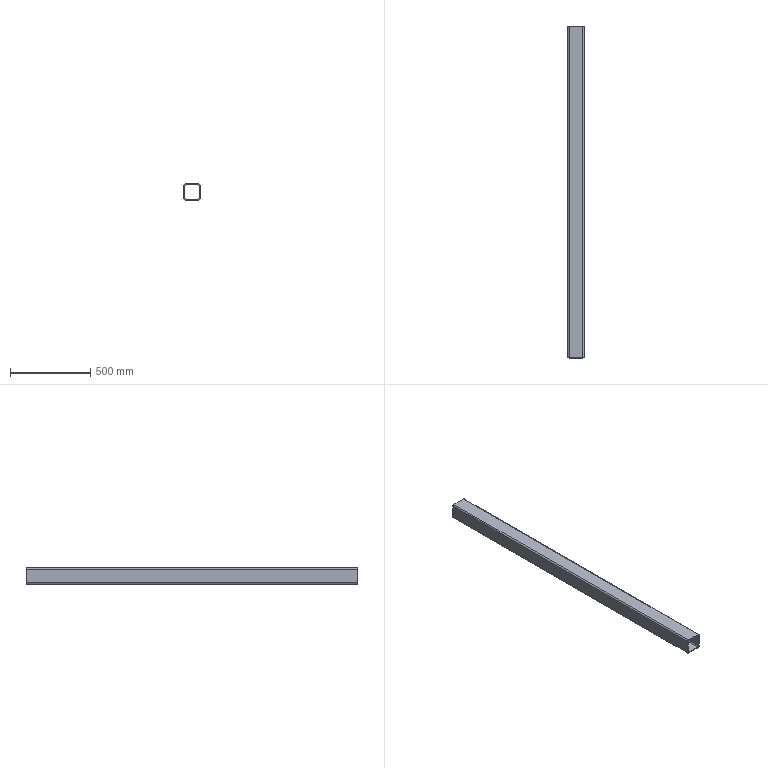Part | SolidWorks | features Extrusion 1 | 1 solid | 18 faces | box 100 x 2070 x 100 mm | volume 4848096 mm3 | plane 10 | cylinder 8 | commonest cylinder face diameters 12.6 x4 15.75 x4
STEP:
#1=CARTESIAN_POINT('',(100.,2070.,-90.6));
#2=VERTEX_POINT('',#1);
#3=CARTESIAN_POINT('',(92.125,2070.,-98.475));
#4=VERTEX_POINT('',#3);
#5=CARTESIAN_POINT('',(92.125,2070.,-90.6));
#6=DIRECTION('',(0.,1.,0.));
#7=DIRECTION('',(0.,0.,1.));
#8=AXIS2_PLACEMENT_3D('',#5,#6,#7);
#9=CIRCLE('',#8,7.875);
#10=EDGE_CURVE('',#2,#4,#9,.T.);
#11=ORIENTED_EDGE('',*,*,#10,.T.);
#12=CARTESIAN_POINT('',(7.875,2070.,-98.475));
#13=VERTEX_POINT('',#12);
#14=CARTESIAN_POINT('',(92.125,2070.,-98.475));
#15=DIRECTION('',(-1.,0.,0.));
#16=VECTOR('',#15,1000.);
#17=LINE('',#14,#16);
#18=EDGE_CURVE('',#4,#13,#17,.T.);
#19=ORIENTED_EDGE('',*,*,#18,.T.);
#20=CARTESIAN_POINT('',(0.,2070.,-90.6));
#21=VERTEX_POINT('',#20);
#22=CARTESIAN_POINT('',(7.875,2070.,-90.6));
#23=DIRECTION('',(0.,1.,0.));
#24=DIRECTION('',(0.,0.,1.));
#25=AXIS2_PLACEMENT_3D('',#22,#23,#24);
#26=CIRCLE('',#25,7.875);
#27=EDGE_CURVE('',#13,#21,#26,.T.);
#28=ORIENTED_EDGE('',*,*,#27,.T.);
#29=CARTESIAN_POINT('',(0.,2070.,-6.35));
#30=VERTEX_POINT('',#29);
#31=CARTESIAN_POINT('',(0.,2070.,-6.35));
#32=DIRECTION('',(0.,0.,1.));
#33=VECTOR('',#32,1000.);
#34=LINE('',#31,#33);
#35=EDGE_CURVE('',#21,#30,#34,.T.);
#36=ORIENTED_EDGE('',*,*,#35,.T.);
#37=CARTESIAN_POINT('',(7.875,2070.,1.525));
#38=VERTEX_POINT('',#37);
#39=CARTESIAN_POINT('',(7.875,2070.,-6.35));
#40=DIRECTION('',(0.,1.,0.));
#41=DIRECTION('',(0.,0.,1.));
#42=AXIS2_PLACEMENT_3D('',#39,#40,#41);
#43=CIRCLE('',#42,7.875);
#44=EDGE_CURVE('',#30,#38,#43,.T.);
#45=ORIENTED_EDGE('',*,*,#44,.T.);
#46=CARTESIAN_POINT('',(92.125,2070.,1.525));
#47=VERTEX_POINT('',#46);
#48=CARTESIAN_POINT('',(7.875,2070.,1.525));
#49=DIRECTION('',(1.,0.,0.));
#50=VECTOR('',#49,1000.);
#51=LINE('',#48,#50);
#52=EDGE_CURVE('',#38,#47,#51,.T.);
#53=ORIENTED_EDGE('',*,*,#52,.T.);
#54=CARTESIAN_POINT('',(100.,2070.,-6.35));
#55=VERTEX_POINT('',#54);
#56=CARTESIAN_POINT('',(92.125,2070.,-6.35));
#57=DIRECTION('',(0.,1.,0.));
#58=DIRECTION('',(0.,0.,1.));
#59=AXIS2_PLACEMENT_3D('',#56,#57,#58);
#60=CIRCLE('',#59,7.875);
#61=EDGE_CURVE('',#47,#55,#60,.T.);
#62=ORIENTED_EDGE('',*,*,#61,.T.);
#63=CARTESIAN_POINT('',(100.,2070.,-90.6));
#64=DIRECTION('',(0.,0.,-1.));
#65=VECTOR('',#64,1000.);
#66=LINE('',#63,#65);
#67=EDGE_CURVE('',#55,#2,#66,.T.);
#68=ORIENTED_EDGE('',*,*,#67,.T.);
#69=EDGE_LOOP('',(#11,#19,#28,#36,#45,#53,#62,#68));
#70=FACE_OUTER_BOUND('',#69,.T.);
#71=CARTESIAN_POINT('',(6.3,2070.,-85.875));
#72=VERTEX_POINT('',#71);
#73=CARTESIAN_POINT('',(6.3,2070.,-11.075));
#74=VERTEX_POINT('',#73);
#75=CARTESIAN_POINT('',(6.3,2070.,-11.075));
#76=DIRECTION('',(0.,0.,1.));
#77=VECTOR('',#76,1000.);
#78=LINE('',#75,#77);
#79=EDGE_CURVE('',#72,#74,#78,.T.);
#80=ORIENTED_EDGE('',*,*,#79,.F.);
#81=CARTESIAN_POINT('',(12.6,2070.,-92.175));
#82=VERTEX_POINT('',#81);
#83=CARTESIAN_POINT('',(12.6,2070.,-85.875));
#84=DIRECTION('',(0.,1.,0.));
#85=DIRECTION('',(0.,0.,1.));
#86=AXIS2_PLACEMENT_3D('',#83,#84,#85);
#87=CIRCLE('',#86,6.3);
#88=EDGE_CURVE('',#82,#72,#87,.T.);
#89=ORIENTED_EDGE('',*,*,#88,.F.);
#90=CARTESIAN_POINT('',(87.4,2070.,-92.175));
#91=VERTEX_POINT('',#90);
#92=CARTESIAN_POINT('',(87.4,2070.,-92.175));
#93=DIRECTION('',(-1.,0.,0.));
#94=VECTOR('',#93,1000.);
#95=LINE('',#92,#94);
#96=EDGE_CURVE('',#91,#82,#95,.T.);
#97=ORIENTED_EDGE('',*,*,#96,.F.);
#98=CARTESIAN_POINT('',(93.7,2070.,-85.875));
#99=VERTEX_POINT('',#98);
#100=CARTESIAN_POINT('',(87.4,2070.,-85.875));
#101=DIRECTION('',(0.,1.,0.));
#102=DIRECTION('',(0.,0.,1.));
#103=AXIS2_PLACEMENT_3D('',#100,#101,#102);
#104=CIRCLE('',#103,6.3);
#105=EDGE_CURVE('',#99,#91,#104,.T.);
#106=ORIENTED_EDGE('',*,*,#105,.F.);
#107=CARTESIAN_POINT('',(93.7,2070.,-11.075));
#108=VERTEX_POINT('',#107);
#109=CARTESIAN_POINT('',(93.7,2070.,-85.875));
#110=DIRECTION('',(0.,0.,-1.));
#111=VECTOR('',#110,1000.);
#112=LINE('',#109,#111);
#113=EDGE_CURVE('',#108,#99,#112,.T.);
#114=ORIENTED_EDGE('',*,*,#113,.F.);
#115=CARTESIAN_POINT('',(87.4,2070.,-4.775));
#116=VERTEX_POINT('',#115);
#117=CARTESIAN_POINT('',(87.4,2070.,-11.075));
#118=DIRECTION('',(0.,1.,0.));
#119=DIRECTION('',(0.,0.,1.));
#120=AXIS2_PLACEMENT_3D('',#117,#118,#119);
#121=CIRCLE('',#120,6.3);
#122=EDGE_CURVE('',#116,#108,#121,.T.);
#123=ORIENTED_EDGE('',*,*,#122,.F.);
#124=CARTESIAN_POINT('',(12.6,2070.,-4.775));
#125=VERTEX_POINT('',#124);
#126=CARTESIAN_POINT('',(12.6,2070.,-4.775));
#127=DIRECTION('',(1.,0.,0.));
#128=VECTOR('',#127,1000.);
#129=LINE('',#126,#128);
#130=EDGE_CURVE('',#125,#116,#129,.T.);
#131=ORIENTED_EDGE('',*,*,#130,.F.);
#132=CARTESIAN_POINT('',(12.6,2070.,-11.075));
#133=DIRECTION('',(0.,1.,0.));
#134=DIRECTION('',(0.,0.,1.));
#135=AXIS2_PLACEMENT_3D('',#132,#133,#134);
#136=CIRCLE('',#135,6.3);
#137=EDGE_CURVE('',#74,#125,#136,.T.);
#138=ORIENTED_EDGE('',*,*,#137,.F.);
#139=EDGE_LOOP('',(#80,#89,#97,#106,#114,#123,#131,#138));
#140=FACE_BOUND('',#139,.T.);
#141=CARTESIAN_POINT('',(92.125,2070.,-90.6));
#142=DIRECTION('',(0.,1.,0.));
#143=DIRECTION('',(0.,0.,1.));
#144=AXIS2_PLACEMENT_3D('',#141,#142,#143);
#145=PLANE('',#144);
#146=ADVANCED_FACE('',(#70,#140),#145,.T.);
#147=CARTESIAN_POINT('',(100.,0.,-90.6));
#148=VERTEX_POINT('',#147);
#149=CARTESIAN_POINT('',(92.125,0.,-98.475));
#150=VERTEX_POINT('',#149);
#151=CARTESIAN_POINT('',(92.125,0.,-90.6));
#152=DIRECTION('',(0.,1.,0.));
#153=DIRECTION('',(0.,0.,1.));
#154=AXIS2_PLACEMENT_3D('',#151,#152,#153);
#155=CIRCLE('',#154,7.875);
#156=EDGE_CURVE('',#148,#150,#155,.T.);
#157=ORIENTED_EDGE('',*,*,#156,.F.);
#158=CARTESIAN_POINT('',(100.,0.,-6.35));
#159=VERTEX_POINT('',#158);
#160=CARTESIAN_POINT('',(100.,0.,-90.6));
#161=DIRECTION('',(0.,0.,-1.));
#162=VECTOR('',#161,1000.);
#163=LINE('',#160,#162);
#164=EDGE_CURVE('',#159,#148,#163,.T.);
#165=ORIENTED_EDGE('',*,*,#164,.F.);
#166=CARTESIAN_POINT('',(92.125,0.,1.525));
#167=VERTEX_POINT('',#166);
#168=CARTESIAN_POINT('',(92.125,0.,-6.35));
#169=DIRECTION('',(0.,1.,0.));
#170=DIRECTION('',(0.,0.,1.));
#171=AXIS2_PLACEMENT_3D('',#168,#169,#170);
#172=CIRCLE('',#171,7.875);
#173=EDGE_CURVE('',#167,#159,#172,.T.);
#174=ORIENTED_EDGE('',*,*,#173,.F.);
#175=CARTESIAN_POINT('',(7.875,0.,1.525));
#176=VERTEX_POINT('',#175);
#177=CARTESIAN_POINT('',(7.875,0.,1.525));
#178=DIRECTION('',(1.,0.,0.));
#179=VECTOR('',#178,1000.);
#180=LINE('',#177,#179);
#181=EDGE_CURVE('',#176,#167,#180,.T.);
#182=ORIENTED_EDGE('',*,*,#181,.F.);
#183=CARTESIAN_POINT('',(0.,0.,-6.35));
#184=VERTEX_POINT('',#183);
#185=CARTESIAN_POINT('',(7.875,0.,-6.35));
#186=DIRECTION('',(0.,1.,0.));
#187=DIRECTION('',(0.,0.,1.));
#188=AXIS2_PLACEMENT_3D('',#185,#186,#187);
#189=CIRCLE('',#188,7.875);
#190=EDGE_CURVE('',#184,#176,#189,.T.);
#191=ORIENTED_EDGE('',*,*,#190,.F.);
#192=CARTESIAN_POINT('',(0.,0.,-90.6));
#193=VERTEX_POINT('',#192);
#194=CARTESIAN_POINT('',(0.,0.,-6.35));
#195=DIRECTION('',(0.,0.,1.));
#196=VECTOR('',#195,1000.);
#197=LINE('',#194,#196);
#198=EDGE_CURVE('',#193,#184,#197,.T.);
#199=ORIENTED_EDGE('',*,*,#198,.F.);
#200=CARTESIAN_POINT('',(7.875,0.,-98.475));
#201=VERTEX_POINT('',#200);
#202=CARTESIAN_POINT('',(7.875,0.,-90.6));
#203=DIRECTION('',(0.,1.,0.));
#204=DIRECTION('',(0.,0.,1.));
#205=AXIS2_PLACEMENT_3D('',#202,#203,#204);
#206=CIRCLE('',#205,7.875);
#207=EDGE_CURVE('',#201,#193,#206,.T.);
#208=ORIENTED_EDGE('',*,*,#207,.F.);
#209=CARTESIAN_POINT('',(92.125,0.,-98.475));
#210=DIRECTION('',(-1.,0.,0.));
#211=VECTOR('',#210,1000.);
#212=LINE('',#209,#211);
#213=EDGE_CURVE('',#150,#201,#212,.T.);
#214=ORIENTED_EDGE('',*,*,#213,.F.);
#215=EDGE_LOOP('',(#157,#165,#174,#182,#191,#199,#208,#214));
#216=FACE_OUTER_BOUND('',#215,.T.);
#217=CARTESIAN_POINT('',(12.6,0.,-92.175));
#218=VERTEX_POINT('',#217);
#219=CARTESIAN_POINT('',(6.3,0.,-85.875));
#220=VERTEX_POINT('',#219);
#221=CARTESIAN_POINT('',(12.6,0.,-85.875));
#222=DIRECTION('',(0.,1.,0.));
#223=DIRECTION('',(0.,0.,1.));
#224=AXIS2_PLACEMENT_3D('',#221,#222,#223);
#225=CIRCLE('',#224,6.3);
#226=EDGE_CURVE('',#218,#220,#225,.T.);
#227=ORIENTED_EDGE('',*,*,#226,.T.);
#228=CARTESIAN_POINT('',(6.3,0.,-11.075));
#229=VERTEX_POINT('',#228);
#230=CARTESIAN_POINT('',(6.3,0.,-11.075));
#231=DIRECTION('',(0.,0.,1.));
#232=VECTOR('',#231,1000.);
#233=LINE('',#230,#232);
#234=EDGE_CURVE('',#220,#229,#233,.T.);
#235=ORIENTED_EDGE('',*,*,#234,.T.);
#236=CARTESIAN_POINT('',(12.6,0.,-4.775));
#237=VERTEX_POINT('',#236);
#238=CARTESIAN_POINT('',(12.6,0.,-11.075));
#239=DIRECTION('',(0.,1.,0.));
#240=DIRECTION('',(0.,0.,1.));
#241=AXIS2_PLACEMENT_3D('',#238,#239,#240);
#242=CIRCLE('',#241,6.3);
#243=EDGE_CURVE('',#229,#237,#242,.T.);
#244=ORIENTED_EDGE('',*,*,#243,.T.);
#245=CARTESIAN_POINT('',(87.4,0.,-4.775));
#246=VERTEX_POINT('',#245);
#247=CARTESIAN_POINT('',(12.6,0.,-4.775));
#248=DIRECTION('',(1.,0.,0.));
#249=VECTOR('',#248,1000.);
#250=LINE('',#247,#249);
#251=EDGE_CURVE('',#237,#246,#250,.T.);
#252=ORIENTED_EDGE('',*,*,#251,.T.);
#253=CARTESIAN_POINT('',(93.7,0.,-11.075));
#254=VERTEX_POINT('',#253);
#255=CARTESIAN_POINT('',(87.4,0.,-11.075));
#256=DIRECTION('',(0.,1.,0.));
#257=DIRECTION('',(0.,0.,1.));
#258=AXIS2_PLACEMENT_3D('',#255,#256,#257);
#259=CIRCLE('',#258,6.3);
#260=EDGE_CURVE('',#246,#254,#259,.T.);
#261=ORIENTED_EDGE('',*,*,#260,.T.);
#262=CARTESIAN_POINT('',(93.7,0.,-85.875));
#263=VERTEX_POINT('',#262);
#264=CARTESIAN_POINT('',(93.7,0.,-85.875));
#265=DIRECTION('',(0.,0.,-1.));
#266=VECTOR('',#265,1000.);
#267=LINE('',#264,#266);
#268=EDGE_CURVE('',#254,#263,#267,.T.);
#269=ORIENTED_EDGE('',*,*,#268,.T.);
#270=CARTESIAN_POINT('',(87.4,0.,-92.175));
#271=VERTEX_POINT('',#270);
#272=CARTESIAN_POINT('',(87.4,0.,-85.875));
#273=DIRECTION('',(0.,1.,0.));
#274=DIRECTION('',(0.,0.,1.));
#275=AXIS2_PLACEMENT_3D('',#272,#273,#274);
#276=CIRCLE('',#275,6.3);
#277=EDGE_CURVE('',#263,#271,#276,.T.);
#278=ORIENTED_EDGE('',*,*,#277,.T.);
#279=CARTESIAN_POINT('',(87.4,0.,-92.175));
#280=DIRECTION('',(-1.,0.,0.));
#281=VECTOR('',#280,1000.);
#282=LINE('',#279,#281);
#283=EDGE_CURVE('',#271,#218,#282,.T.);
#284=ORIENTED_EDGE('',*,*,#283,.T.);
#285=EDGE_LOOP('',(#227,#235,#244,#252,#261,#269,#278,#284));
#286=FACE_BOUND('',#285,.T.);
#287=CARTESIAN_POINT('',(92.125,0.,-90.6));
#288=DIRECTION('',(0.,1.,0.));
#289=DIRECTION('',(0.,0.,1.));
#290=AXIS2_PLACEMENT_3D('',#287,#288,#289);
#291=PLANE('',#290);
#292=ADVANCED_FACE('',(#216,#286),#291,.F.);
#293=ORIENTED_EDGE('',*,*,#156,.T.);
#294=CARTESIAN_POINT('',(92.125,2070.,-98.475));
#295=DIRECTION('',(0.,-1.,0.));
#296=VECTOR('',#295,1000.);
#297=LINE('',#294,#296);
#298=EDGE_CURVE('',#4,#150,#297,.T.);
#299=ORIENTED_EDGE('',*,*,#298,.F.);
#300=ORIENTED_EDGE('',*,*,#10,.F.);
#301=CARTESIAN_POINT('',(100.,2070.,-90.6));
#302=DIRECTION('',(0.,-1.,0.));
#303=VECTOR('',#302,1000.);
#304=LINE('',#301,#303);
#305=EDGE_CURVE('',#2,#148,#304,.T.);
#306=ORIENTED_EDGE('',*,*,#305,.T.);
#307=EDGE_LOOP('',(#293,#299,#300,#306));
#308=FACE_OUTER_BOUND('',#307,.T.);
#309=CARTESIAN_POINT('',(92.125,2070.,-90.6));
#310=DIRECTION('',(0.,-1.,0.));
#311=DIRECTION('',(0.,0.,-1.));
#312=AXIS2_PLACEMENT_3D('',#309,#310,#311);
#313=CYLINDRICAL_SURFACE('',#312,7.875);
#314=ADVANCED_FACE('',(#308),#313,.T.);
#315=ORIENTED_EDGE('',*,*,#213,.T.);
#316=CARTESIAN_POINT('',(7.875,2070.,-98.475));
#317=DIRECTION('',(0.,-1.,0.));
#318=VECTOR('',#317,1000.);
#319=LINE('',#316,#318);
#320=EDGE_CURVE('',#13,#201,#319,.T.);
#321=ORIENTED_EDGE('',*,*,#320,.F.);
#322=ORIENTED_EDGE('',*,*,#18,.F.);
#323=ORIENTED_EDGE('',*,*,#298,.T.);
#324=EDGE_LOOP('',(#315,#321,#322,#323));
#325=FACE_OUTER_BOUND('',#324,.T.);
#326=CARTESIAN_POINT('',(92.125,2070.,-98.475));
#327=DIRECTION('',(0.,0.,1.));
#328=DIRECTION('',(1.,0.,0.));
#329=AXIS2_PLACEMENT_3D('',#326,#327,#328);
#330=PLANE('',#329);
#331=ADVANCED_FACE('',(#325),#330,.F.);
#332=ORIENTED_EDGE('',*,*,#207,.T.);
#333=CARTESIAN_POINT('',(0.,2070.,-90.6));
#334=DIRECTION('',(0.,-1.,0.));
#335=VECTOR('',#334,1000.);
#336=LINE('',#333,#335);
#337=EDGE_CURVE('',#21,#193,#336,.T.);
#338=ORIENTED_EDGE('',*,*,#337,.F.);
#339=ORIENTED_EDGE('',*,*,#27,.F.);
#340=ORIENTED_EDGE('',*,*,#320,.T.);
#341=EDGE_LOOP('',(#332,#338,#339,#340));
#342=FACE_OUTER_BOUND('',#341,.T.);
#343=CARTESIAN_POINT('',(7.875,2070.,-90.6));
#344=DIRECTION('',(0.,-1.,0.));
#345=DIRECTION('',(0.,0.,-1.));
#346=AXIS2_PLACEMENT_3D('',#343,#344,#345);
#347=CYLINDRICAL_SURFACE('',#346,7.875);
#348=ADVANCED_FACE('',(#342),#347,.T.);
#349=ORIENTED_EDGE('',*,*,#198,.T.);
#350=CARTESIAN_POINT('',(0.,2070.,-6.35));
#351=DIRECTION('',(0.,-1.,0.));
#352=VECTOR('',#351,1000.);
#353=LINE('',#350,#352);
#354=EDGE_CURVE('',#30,#184,#353,.T.);
#355=ORIENTED_EDGE('',*,*,#354,.F.);
#356=ORIENTED_EDGE('',*,*,#35,.F.);
#357=ORIENTED_EDGE('',*,*,#337,.T.);
#358=EDGE_LOOP('',(#349,#355,#356,#357));
#359=FACE_OUTER_BOUND('',#358,.T.);
#360=CARTESIAN_POINT('',(0.,2070.,-6.35));
#361=DIRECTION('',(1.,0.,0.));
#362=DIRECTION('',(0.,0.,-1.));
#363=AXIS2_PLACEMENT_3D('',#360,#361,#362);
#364=PLANE('',#363);
#365=ADVANCED_FACE('',(#359),#364,.F.);
#366=ORIENTED_EDGE('',*,*,#190,.T.);
#367=CARTESIAN_POINT('',(7.875,2070.,1.525));
#368=DIRECTION('',(0.,-1.,0.));
#369=VECTOR('',#368,1000.);
#370=LINE('',#367,#369);
#371=EDGE_CURVE('',#38,#176,#370,.T.);
#372=ORIENTED_EDGE('',*,*,#371,.F.);
#373=ORIENTED_EDGE('',*,*,#44,.F.);
#374=ORIENTED_EDGE('',*,*,#354,.T.);
#375=EDGE_LOOP('',(#366,#372,#373,#374));
#376=FACE_OUTER_BOUND('',#375,.T.);
#377=CARTESIAN_POINT('',(7.875,2070.,-6.35));
#378=DIRECTION('',(0.,-1.,0.));
#379=DIRECTION('',(0.,0.,-1.));
#380=AXIS2_PLACEMENT_3D('',#377,#378,#379);
#381=CYLINDRICAL_SURFACE('',#380,7.875);
#382=ADVANCED_FACE('',(#376),#381,.T.);
#383=ORIENTED_EDGE('',*,*,#181,.T.);
#384=CARTESIAN_POINT('',(92.125,2070.,1.525));
#385=DIRECTION('',(0.,-1.,0.));
#386=VECTOR('',#385,1000.);
#387=LINE('',#384,#386);
#388=EDGE_CURVE('',#47,#167,#387,.T.);
#389=ORIENTED_EDGE('',*,*,#388,.F.);
#390=ORIENTED_EDGE('',*,*,#52,.F.);
#391=ORIENTED_EDGE('',*,*,#371,.T.);
#392=EDGE_LOOP('',(#383,#389,#390,#391));
#393=FACE_OUTER_BOUND('',#392,.T.);
#394=CARTESIAN_POINT('',(7.875,2070.,1.525));
#395=DIRECTION('',(0.,0.,-1.));
#396=DIRECTION('',(-1.,0.,0.));
#397=AXIS2_PLACEMENT_3D('',#394,#395,#396);
#398=PLANE('',#397);
#399=ADVANCED_FACE('',(#393),#398,.F.);
#400=ORIENTED_EDGE('',*,*,#173,.T.);
#401=CARTESIAN_POINT('',(100.,2070.,-6.35));
#402=DIRECTION('',(0.,-1.,0.));
#403=VECTOR('',#402,1000.);
#404=LINE('',#401,#403);
#405=EDGE_CURVE('',#55,#159,#404,.T.);
#406=ORIENTED_EDGE('',*,*,#405,.F.);
#407=ORIENTED_EDGE('',*,*,#61,.F.);
#408=ORIENTED_EDGE('',*,*,#388,.T.);
#409=EDGE_LOOP('',(#400,#406,#407,#408));
#410=FACE_OUTER_BOUND('',#409,.T.);
#411=CARTESIAN_POINT('',(92.125,2070.,-6.35));
#412=DIRECTION('',(0.,-1.,0.));
#413=DIRECTION('',(0.,0.,-1.));
#414=AXIS2_PLACEMENT_3D('',#411,#412,#413);
#415=CYLINDRICAL_SURFACE('',#414,7.875);
#416=ADVANCED_FACE('',(#410),#415,.T.);
#417=ORIENTED_EDGE('',*,*,#164,.T.);
#418=ORIENTED_EDGE('',*,*,#305,.F.);
#419=ORIENTED_EDGE('',*,*,#67,.F.);
#420=ORIENTED_EDGE('',*,*,#405,.T.);
#421=EDGE_LOOP('',(#417,#418,#419,#420));
#422=FACE_OUTER_BOUND('',#421,.T.);
#423=CARTESIAN_POINT('',(100.,2070.,-90.6));
#424=DIRECTION('',(-1.,0.,0.));
#425=DIRECTION('',(0.,0.,1.));
#426=AXIS2_PLACEMENT_3D('',#423,#424,#425);
#427=PLANE('',#426);
#428=ADVANCED_FACE('',(#422),#427,.F.);
#429=ORIENTED_EDGE('',*,*,#226,.F.);
#430=CARTESIAN_POINT('',(12.6,2070.,-92.175));
#431=DIRECTION('',(0.,-1.,0.));
#432=VECTOR('',#431,1000.);
#433=LINE('',#430,#432);
#434=EDGE_CURVE('',#82,#218,#433,.T.);
#435=ORIENTED_EDGE('',*,*,#434,.F.);
#436=ORIENTED_EDGE('',*,*,#88,.T.);
#437=CARTESIAN_POINT('',(6.3,2070.,-85.875));
#438=DIRECTION('',(0.,-1.,0.));
#439=VECTOR('',#438,1000.);
#440=LINE('',#437,#439);
#441=EDGE_CURVE('',#72,#220,#440,.T.);
#442=ORIENTED_EDGE('',*,*,#441,.T.);
#443=EDGE_LOOP('',(#429,#435,#436,#442));
#444=FACE_OUTER_BOUND('',#443,.T.);
#445=CARTESIAN_POINT('',(12.6,2070.,-85.875));
#446=DIRECTION('',(0.,-1.,0.));
#447=DIRECTION('',(0.,0.,-1.));
#448=AXIS2_PLACEMENT_3D('',#445,#446,#447);
#449=CYLINDRICAL_SURFACE('',#448,6.3);
#450=ADVANCED_FACE('',(#444),#449,.F.);
#451=ORIENTED_EDGE('',*,*,#234,.F.);
#452=ORIENTED_EDGE('',*,*,#441,.F.);
#453=ORIENTED_EDGE('',*,*,#79,.T.);
#454=CARTESIAN_POINT('',(6.3,2070.,-11.075));
#455=DIRECTION('',(0.,-1.,0.));
#456=VECTOR('',#455,1000.);
#457=LINE('',#454,#456);
#458=EDGE_CURVE('',#74,#229,#457,.T.);
#459=ORIENTED_EDGE('',*,*,#458,.T.);
#460=EDGE_LOOP('',(#451,#452,#453,#459));
#461=FACE_OUTER_BOUND('',#460,.T.);
#462=CARTESIAN_POINT('',(6.3,2070.,-11.075));
#463=DIRECTION('',(1.,0.,0.));
#464=DIRECTION('',(0.,0.,-1.));
#465=AXIS2_PLACEMENT_3D('',#462,#463,#464);
#466=PLANE('',#465);
#467=ADVANCED_FACE('',(#461),#466,.T.);
#468=ORIENTED_EDGE('',*,*,#243,.F.);
#469=ORIENTED_EDGE('',*,*,#458,.F.);
#470=ORIENTED_EDGE('',*,*,#137,.T.);
#471=CARTESIAN_POINT('',(12.6,2070.,-4.775));
#472=DIRECTION('',(0.,-1.,0.));
#473=VECTOR('',#472,1000.);
#474=LINE('',#471,#473);
#475=EDGE_CURVE('',#125,#237,#474,.T.);
#476=ORIENTED_EDGE('',*,*,#475,.T.);
#477=EDGE_LOOP('',(#468,#469,#470,#476));
#478=FACE_OUTER_BOUND('',#477,.T.);
#479=CARTESIAN_POINT('',(12.6,2070.,-11.075));
#480=DIRECTION('',(0.,-1.,0.));
#481=DIRECTION('',(0.,0.,-1.));
#482=AXIS2_PLACEMENT_3D('',#479,#480,#481);
#483=CYLINDRICAL_SURFACE('',#482,6.3);
#484=ADVANCED_FACE('',(#478),#483,.F.);
#485=ORIENTED_EDGE('',*,*,#251,.F.);
#486=ORIENTED_EDGE('',*,*,#475,.F.);
#487=ORIENTED_EDGE('',*,*,#130,.T.);
#488=CARTESIAN_POINT('',(87.4,2070.,-4.775));
#489=DIRECTION('',(0.,-1.,0.));
#490=VECTOR('',#489,1000.);
#491=LINE('',#488,#490);
#492=EDGE_CURVE('',#116,#246,#491,.T.);
#493=ORIENTED_EDGE('',*,*,#492,.T.);
#494=EDGE_LOOP('',(#485,#486,#487,#493));
#495=FACE_OUTER_BOUND('',#494,.T.);
#496=CARTESIAN_POINT('',(12.6,2070.,-4.775));
#497=DIRECTION('',(0.,0.,-1.));
#498=DIRECTION('',(-1.,0.,0.));
#499=AXIS2_PLACEMENT_3D('',#496,#497,#498);
#500=PLANE('',#499);
#501=ADVANCED_FACE('',(#495),#500,.T.);
#502=ORIENTED_EDGE('',*,*,#260,.F.);
#503=ORIENTED_EDGE('',*,*,#492,.F.);
#504=ORIENTED_EDGE('',*,*,#122,.T.);
#505=CARTESIAN_POINT('',(93.7,2070.,-11.075));
#506=DIRECTION('',(0.,-1.,0.));
#507=VECTOR('',#506,1000.);
#508=LINE('',#505,#507);
#509=EDGE_CURVE('',#108,#254,#508,.T.);
#510=ORIENTED_EDGE('',*,*,#509,.T.);
#511=EDGE_LOOP('',(#502,#503,#504,#510));
#512=FACE_OUTER_BOUND('',#511,.T.);
#513=CARTESIAN_POINT('',(87.4,2070.,-11.075));
#514=DIRECTION('',(0.,-1.,0.));
#515=DIRECTION('',(0.,0.,-1.));
#516=AXIS2_PLACEMENT_3D('',#513,#514,#515);
#517=CYLINDRICAL_SURFACE('',#516,6.3);
#518=ADVANCED_FACE('',(#512),#517,.F.);
#519=ORIENTED_EDGE('',*,*,#268,.F.);
#520=ORIENTED_EDGE('',*,*,#509,.F.);
#521=ORIENTED_EDGE('',*,*,#113,.T.);
#522=CARTESIAN_POINT('',(93.7,2070.,-85.875));
#523=DIRECTION('',(0.,-1.,0.));
#524=VECTOR('',#523,1000.);
#525=LINE('',#522,#524);
#526=EDGE_CURVE('',#99,#263,#525,.T.);
#527=ORIENTED_EDGE('',*,*,#526,.T.);
#528=EDGE_LOOP('',(#519,#520,#521,#527));
#529=FACE_OUTER_BOUND('',#528,.T.);
#530=CARTESIAN_POINT('',(93.7,2070.,-85.875));
#531=DIRECTION('',(-1.,0.,0.));
#532=DIRECTION('',(0.,0.,1.));
#533=AXIS2_PLACEMENT_3D('',#530,#531,#532);
#534=PLANE('',#533);
#535=ADVANCED_FACE('',(#529),#534,.T.);
#536=ORIENTED_EDGE('',*,*,#277,.F.);
#537=ORIENTED_EDGE('',*,*,#526,.F.);
#538=ORIENTED_EDGE('',*,*,#105,.T.);
#539=CARTESIAN_POINT('',(87.4,2070.,-92.175));
#540=DIRECTION('',(0.,-1.,0.));
#541=VECTOR('',#540,1000.);
#542=LINE('',#539,#541);
#543=EDGE_CURVE('',#91,#271,#542,.T.);
#544=ORIENTED_EDGE('',*,*,#543,.T.);
#545=EDGE_LOOP('',(#536,#537,#538,#544));
#546=FACE_OUTER_BOUND('',#545,.T.);
#547=CARTESIAN_POINT('',(87.4,2070.,-85.875));
#548=DIRECTION('',(0.,-1.,0.));
#549=DIRECTION('',(0.,0.,-1.));
#550=AXIS2_PLACEMENT_3D('',#547,#548,#549);
#551=CYLINDRICAL_SURFACE('',#550,6.3);
#552=ADVANCED_FACE('',(#546),#551,.F.);
#553=ORIENTED_EDGE('',*,*,#283,.F.);
#554=ORIENTED_EDGE('',*,*,#543,.F.);
#555=ORIENTED_EDGE('',*,*,#96,.T.);
#556=ORIENTED_EDGE('',*,*,#434,.T.);
#557=EDGE_LOOP('',(#553,#554,#555,#556));
#558=FACE_OUTER_BOUND('',#557,.T.);
#559=CARTESIAN_POINT('',(87.4,2070.,-92.175));
#560=DIRECTION('',(0.,0.,1.));
#561=DIRECTION('',(1.,0.,0.));
#562=AXIS2_PLACEMENT_3D('',#559,#560,#561);
#563=PLANE('',#562);
#564=ADVANCED_FACE('',(#558),#563,.T.);
#565=CLOSED_SHELL('',(#146,#292,#314,#331,#348,#365,#382,#399,#416,#428,#450,#467,#484,#501,#518,#535,#552,#564));
#566=MANIFOLD_SOLID_BREP('',#565);
#567=CARTESIAN_POINT('',(0.,0.,0.));
#568=DIRECTION('',(0.,0.,1.));
#569=DIRECTION('',(1.,0.,0.));
#570=AXIS2_PLACEMENT_3D('',#567,#568,#569);
#571=(LENGTH_UNIT()NAMED_UNIT(*)SI_UNIT(.MILLI.,.METRE.));
#572=UNCERTAINTY_MEASURE_WITH_UNIT(LENGTH_MEASURE(0.00001),#571,'','');
#573=(NAMED_UNIT(*)PLANE_ANGLE_UNIT()SI_UNIT($,.RADIAN.));
#574=(NAMED_UNIT(*)SI_UNIT($,.STERADIAN.)SOLID_ANGLE_UNIT());
#575=(GEOMETRIC_REPRESENTATION_CONTEXT(3)GLOBAL_UNCERTAINTY_ASSIGNED_CONTEXT((#572))GLOBAL_UNIT_ASSIGNED_CONTEXT((#571,#573,#574))REPRESENTATION_CONTEXT('',''));
#576=ADVANCED_BREP_SHAPE_REPRESENTATION('',(#566,#570),#575);